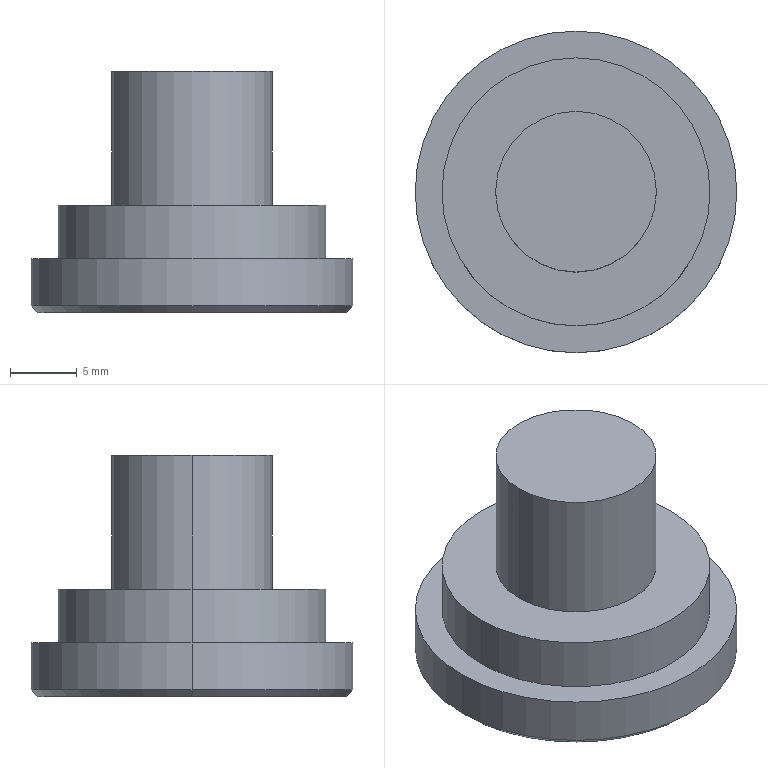Part | SolidWorks | features ICE 2, Chamfer 1, Extrusion 1 | 1 solid | 12 faces | box 24 x 24 x 18 mm | volume 4188 mm3 | cylinder 6 | plane 4 | cone 2 | commonest cylinder face diameters 12 x2 20 x2 24 x2
STEP:
#1=CARTESIAN_POINT('',(-11.5,0.,0.));
#2=VERTEX_POINT('',#1);
#3=CARTESIAN_POINT('',(11.5,0.,0.));
#4=VERTEX_POINT('',#3);
#5=CARTESIAN_POINT('',(0.,0.,0.));
#6=DIRECTION('',(0.,0.,-1.));
#7=DIRECTION('',(1.,0.,0.));
#8=AXIS2_PLACEMENT_3D('',#5,#6,#7);
#9=CIRCLE('',#8,11.5);
#10=EDGE_CURVE('',#2,#4,#9,.T.);
#11=ORIENTED_EDGE('',*,*,#10,.F.);
#12=CARTESIAN_POINT('',(-12.,0.,0.5));
#13=VERTEX_POINT('',#12);
#14=CARTESIAN_POINT('',(-12.,0.,0.5));
#15=DIRECTION('',(-0.7071,0.,0.7071));
#16=VECTOR('',#15,1000.);
#17=LINE('',#14,#16);
#18=EDGE_CURVE('',#2,#13,#17,.T.);
#19=ORIENTED_EDGE('',*,*,#18,.T.);
#20=CARTESIAN_POINT('',(12.,0.,0.5));
#21=VERTEX_POINT('',#20);
#22=CARTESIAN_POINT('',(0.,0.,0.5));
#23=DIRECTION('',(0.,0.,1.));
#24=DIRECTION('',(1.,0.,0.));
#25=AXIS2_PLACEMENT_3D('',#22,#23,#24);
#26=CIRCLE('',#25,12.);
#27=EDGE_CURVE('',#21,#13,#26,.T.);
#28=ORIENTED_EDGE('',*,*,#27,.F.);
#29=CARTESIAN_POINT('',(12.,0.,0.5));
#30=DIRECTION('',(0.7071,0.,0.7071));
#31=VECTOR('',#30,1000.);
#32=LINE('',#29,#31);
#33=EDGE_CURVE('',#4,#21,#32,.T.);
#34=ORIENTED_EDGE('',*,*,#33,.F.);
#35=EDGE_LOOP('',(#11,#19,#28,#34));
#36=FACE_OUTER_BOUND('',#35,.T.);
#37=CARTESIAN_POINT('',(0.,0.,0.5));
#38=DIRECTION('',(0.,0.,1.));
#39=DIRECTION('',(1.,0.,0.));
#40=AXIS2_PLACEMENT_3D('',#37,#38,#39);
#41=CONICAL_SURFACE('',#40,12.,0.7854);
#42=ADVANCED_FACE('',(#36),#41,.T.);
#43=CARTESIAN_POINT('',(12.,0.,4.));
#44=VERTEX_POINT('',#43);
#45=CARTESIAN_POINT('',(-12.,0.,4.));
#46=VERTEX_POINT('',#45);
#47=CARTESIAN_POINT('',(0.,0.,4.));
#48=DIRECTION('',(0.,0.,1.));
#49=DIRECTION('',(1.,0.,0.));
#50=AXIS2_PLACEMENT_3D('',#47,#48,#49);
#51=CIRCLE('',#50,12.);
#52=EDGE_CURVE('',#44,#46,#51,.T.);
#53=ORIENTED_EDGE('',*,*,#52,.F.);
#54=CARTESIAN_POINT('',(12.,0.,4.));
#55=DIRECTION('',(0.,0.,-1.));
#56=VECTOR('',#55,1000.);
#57=LINE('',#54,#56);
#58=EDGE_CURVE('',#44,#21,#57,.T.);
#59=ORIENTED_EDGE('',*,*,#58,.T.);
#60=ORIENTED_EDGE('',*,*,#27,.T.);
#61=CARTESIAN_POINT('',(-12.,0.,4.));
#62=DIRECTION('',(0.,0.,-1.));
#63=VECTOR('',#62,1000.);
#64=LINE('',#61,#63);
#65=EDGE_CURVE('',#46,#13,#64,.T.);
#66=ORIENTED_EDGE('',*,*,#65,.F.);
#67=EDGE_LOOP('',(#53,#59,#60,#66));
#68=FACE_OUTER_BOUND('',#67,.T.);
#69=CARTESIAN_POINT('',(0.,0.,4.));
#70=DIRECTION('',(0.,0.,-1.));
#71=DIRECTION('',(-1.,0.,0.));
#72=AXIS2_PLACEMENT_3D('',#69,#70,#71);
#73=CYLINDRICAL_SURFACE('',#72,12.);
#74=ADVANCED_FACE('',(#68),#73,.T.);
#75=CARTESIAN_POINT('',(10.,0.,8.));
#76=VERTEX_POINT('',#75);
#77=CARTESIAN_POINT('',(-10.,0.,8.));
#78=VERTEX_POINT('',#77);
#79=CARTESIAN_POINT('',(0.,0.,8.));
#80=DIRECTION('',(0.,0.,1.));
#81=DIRECTION('',(1.,0.,0.));
#82=AXIS2_PLACEMENT_3D('',#79,#80,#81);
#83=CIRCLE('',#82,10.);
#84=EDGE_CURVE('',#76,#78,#83,.T.);
#85=ORIENTED_EDGE('',*,*,#84,.F.);
#86=CARTESIAN_POINT('',(10.,0.,4.));
#87=VERTEX_POINT('',#86);
#88=CARTESIAN_POINT('',(10.,0.,8.));
#89=DIRECTION('',(0.,0.,-1.));
#90=VECTOR('',#89,1000.);
#91=LINE('',#88,#90);
#92=EDGE_CURVE('',#76,#87,#91,.T.);
#93=ORIENTED_EDGE('',*,*,#92,.T.);
#94=CARTESIAN_POINT('',(-10.,0.,4.));
#95=VERTEX_POINT('',#94);
#96=CARTESIAN_POINT('',(0.,0.,4.));
#97=DIRECTION('',(0.,0.,1.));
#98=DIRECTION('',(1.,0.,0.));
#99=AXIS2_PLACEMENT_3D('',#96,#97,#98);
#100=CIRCLE('',#99,10.);
#101=EDGE_CURVE('',#87,#95,#100,.T.);
#102=ORIENTED_EDGE('',*,*,#101,.T.);
#103=CARTESIAN_POINT('',(-10.,0.,8.));
#104=DIRECTION('',(0.,0.,-1.));
#105=VECTOR('',#104,1000.);
#106=LINE('',#103,#105);
#107=EDGE_CURVE('',#78,#95,#106,.T.);
#108=ORIENTED_EDGE('',*,*,#107,.F.);
#109=EDGE_LOOP('',(#85,#93,#102,#108));
#110=FACE_OUTER_BOUND('',#109,.T.);
#111=CARTESIAN_POINT('',(0.,0.,8.));
#112=DIRECTION('',(0.,0.,-1.));
#113=DIRECTION('',(-1.,0.,0.));
#114=AXIS2_PLACEMENT_3D('',#111,#112,#113);
#115=CYLINDRICAL_SURFACE('',#114,10.);
#116=ADVANCED_FACE('',(#110),#115,.T.);
#117=CARTESIAN_POINT('',(6.,0.,18.));
#118=VERTEX_POINT('',#117);
#119=CARTESIAN_POINT('',(-6.,0.,18.));
#120=VERTEX_POINT('',#119);
#121=CARTESIAN_POINT('',(0.,0.,18.));
#122=DIRECTION('',(0.,0.,1.));
#123=DIRECTION('',(1.,0.,0.));
#124=AXIS2_PLACEMENT_3D('',#121,#122,#123);
#125=CIRCLE('',#124,6.);
#126=EDGE_CURVE('',#118,#120,#125,.T.);
#127=ORIENTED_EDGE('',*,*,#126,.F.);
#128=CARTESIAN_POINT('',(6.,0.,8.));
#129=VERTEX_POINT('',#128);
#130=CARTESIAN_POINT('',(6.,0.,18.));
#131=DIRECTION('',(0.,0.,-1.));
#132=VECTOR('',#131,1000.);
#133=LINE('',#130,#132);
#134=EDGE_CURVE('',#118,#129,#133,.T.);
#135=ORIENTED_EDGE('',*,*,#134,.T.);
#136=CARTESIAN_POINT('',(-6.,0.,8.));
#137=VERTEX_POINT('',#136);
#138=CARTESIAN_POINT('',(0.,0.,8.));
#139=DIRECTION('',(0.,0.,1.));
#140=DIRECTION('',(1.,0.,0.));
#141=AXIS2_PLACEMENT_3D('',#138,#139,#140);
#142=CIRCLE('',#141,6.);
#143=EDGE_CURVE('',#129,#137,#142,.T.);
#144=ORIENTED_EDGE('',*,*,#143,.T.);
#145=CARTESIAN_POINT('',(-6.,0.,18.));
#146=DIRECTION('',(0.,0.,-1.));
#147=VECTOR('',#146,1000.);
#148=LINE('',#145,#147);
#149=EDGE_CURVE('',#120,#137,#148,.T.);
#150=ORIENTED_EDGE('',*,*,#149,.F.);
#151=EDGE_LOOP('',(#127,#135,#144,#150));
#152=FACE_OUTER_BOUND('',#151,.T.);
#153=CARTESIAN_POINT('',(0.,0.,18.));
#154=DIRECTION('',(0.,0.,-1.));
#155=DIRECTION('',(-1.,0.,0.));
#156=AXIS2_PLACEMENT_3D('',#153,#154,#155);
#157=CYLINDRICAL_SURFACE('',#156,6.);
#158=ADVANCED_FACE('',(#152),#157,.T.);
#159=ORIENTED_EDGE('',*,*,#134,.F.);
#160=CARTESIAN_POINT('',(0.,0.,18.));
#161=DIRECTION('',(0.,0.,1.));
#162=DIRECTION('',(1.,0.,0.));
#163=AXIS2_PLACEMENT_3D('',#160,#161,#162);
#164=CIRCLE('',#163,6.);
#165=EDGE_CURVE('',#120,#118,#164,.T.);
#166=ORIENTED_EDGE('',*,*,#165,.F.);
#167=ORIENTED_EDGE('',*,*,#149,.T.);
#168=CARTESIAN_POINT('',(0.,0.,8.));
#169=DIRECTION('',(0.,0.,1.));
#170=DIRECTION('',(1.,0.,0.));
#171=AXIS2_PLACEMENT_3D('',#168,#169,#170);
#172=CIRCLE('',#171,6.);
#173=EDGE_CURVE('',#137,#129,#172,.T.);
#174=ORIENTED_EDGE('',*,*,#173,.T.);
#175=EDGE_LOOP('',(#159,#166,#167,#174));
#176=FACE_OUTER_BOUND('',#175,.T.);
#177=CARTESIAN_POINT('',(0.,0.,18.));
#178=DIRECTION('',(0.,0.,-1.));
#179=DIRECTION('',(-1.,0.,0.));
#180=AXIS2_PLACEMENT_3D('',#177,#178,#179);
#181=CYLINDRICAL_SURFACE('',#180,6.);
#182=ADVANCED_FACE('',(#176),#181,.T.);
#183=ORIENTED_EDGE('',*,*,#165,.T.);
#184=ORIENTED_EDGE('',*,*,#126,.T.);
#185=EDGE_LOOP('',(#183,#184));
#186=FACE_OUTER_BOUND('',#185,.T.);
#187=CARTESIAN_POINT('',(0.,0.,18.));
#188=DIRECTION('',(0.,0.,1.));
#189=DIRECTION('',(1.,0.,0.));
#190=AXIS2_PLACEMENT_3D('',#187,#188,#189);
#191=PLANE('',#190);
#192=ADVANCED_FACE('',(#186),#191,.T.);
#193=ORIENTED_EDGE('',*,*,#92,.F.);
#194=CARTESIAN_POINT('',(0.,0.,8.));
#195=DIRECTION('',(0.,0.,1.));
#196=DIRECTION('',(1.,0.,0.));
#197=AXIS2_PLACEMENT_3D('',#194,#195,#196);
#198=CIRCLE('',#197,10.);
#199=EDGE_CURVE('',#78,#76,#198,.T.);
#200=ORIENTED_EDGE('',*,*,#199,.F.);
#201=ORIENTED_EDGE('',*,*,#107,.T.);
#202=CARTESIAN_POINT('',(0.,0.,4.));
#203=DIRECTION('',(0.,0.,1.));
#204=DIRECTION('',(1.,0.,0.));
#205=AXIS2_PLACEMENT_3D('',#202,#203,#204);
#206=CIRCLE('',#205,10.);
#207=EDGE_CURVE('',#95,#87,#206,.T.);
#208=ORIENTED_EDGE('',*,*,#207,.T.);
#209=EDGE_LOOP('',(#193,#200,#201,#208));
#210=FACE_OUTER_BOUND('',#209,.T.);
#211=CARTESIAN_POINT('',(0.,0.,8.));
#212=DIRECTION('',(0.,0.,-1.));
#213=DIRECTION('',(-1.,0.,0.));
#214=AXIS2_PLACEMENT_3D('',#211,#212,#213);
#215=CYLINDRICAL_SURFACE('',#214,10.);
#216=ADVANCED_FACE('',(#210),#215,.T.);
#217=ORIENTED_EDGE('',*,*,#173,.F.);
#218=ORIENTED_EDGE('',*,*,#143,.F.);
#219=EDGE_LOOP('',(#217,#218));
#220=FACE_BOUND('',#219,.T.);
#221=ORIENTED_EDGE('',*,*,#199,.T.);
#222=ORIENTED_EDGE('',*,*,#84,.T.);
#223=EDGE_LOOP('',(#221,#222));
#224=FACE_OUTER_BOUND('',#223,.T.);
#225=CARTESIAN_POINT('',(0.,0.,8.));
#226=DIRECTION('',(0.,0.,1.));
#227=DIRECTION('',(1.,0.,0.));
#228=AXIS2_PLACEMENT_3D('',#225,#226,#227);
#229=PLANE('',#228);
#230=ADVANCED_FACE('',(#220,#224),#229,.T.);
#231=ORIENTED_EDGE('',*,*,#58,.F.);
#232=CARTESIAN_POINT('',(0.,0.,4.));
#233=DIRECTION('',(0.,0.,1.));
#234=DIRECTION('',(1.,0.,0.));
#235=AXIS2_PLACEMENT_3D('',#232,#233,#234);
#236=CIRCLE('',#235,12.);
#237=EDGE_CURVE('',#46,#44,#236,.T.);
#238=ORIENTED_EDGE('',*,*,#237,.F.);
#239=ORIENTED_EDGE('',*,*,#65,.T.);
#240=CARTESIAN_POINT('',(0.,0.,0.5));
#241=DIRECTION('',(0.,0.,1.));
#242=DIRECTION('',(1.,0.,0.));
#243=AXIS2_PLACEMENT_3D('',#240,#241,#242);
#244=CIRCLE('',#243,12.);
#245=EDGE_CURVE('',#13,#21,#244,.T.);
#246=ORIENTED_EDGE('',*,*,#245,.T.);
#247=EDGE_LOOP('',(#231,#238,#239,#246));
#248=FACE_OUTER_BOUND('',#247,.T.);
#249=CARTESIAN_POINT('',(0.,0.,4.));
#250=DIRECTION('',(0.,0.,-1.));
#251=DIRECTION('',(-1.,0.,0.));
#252=AXIS2_PLACEMENT_3D('',#249,#250,#251);
#253=CYLINDRICAL_SURFACE('',#252,12.);
#254=ADVANCED_FACE('',(#248),#253,.T.);
#255=ORIENTED_EDGE('',*,*,#207,.F.);
#256=ORIENTED_EDGE('',*,*,#101,.F.);
#257=EDGE_LOOP('',(#255,#256));
#258=FACE_BOUND('',#257,.T.);
#259=ORIENTED_EDGE('',*,*,#237,.T.);
#260=ORIENTED_EDGE('',*,*,#52,.T.);
#261=EDGE_LOOP('',(#259,#260));
#262=FACE_OUTER_BOUND('',#261,.T.);
#263=CARTESIAN_POINT('',(0.,0.,4.));
#264=DIRECTION('',(0.,0.,1.));
#265=DIRECTION('',(1.,0.,0.));
#266=AXIS2_PLACEMENT_3D('',#263,#264,#265);
#267=PLANE('',#266);
#268=ADVANCED_FACE('',(#258,#262),#267,.T.);
#269=CARTESIAN_POINT('',(0.,0.,0.));
#270=DIRECTION('',(0.,0.,-1.));
#271=DIRECTION('',(1.,0.,0.));
#272=AXIS2_PLACEMENT_3D('',#269,#270,#271);
#273=CIRCLE('',#272,11.5);
#274=EDGE_CURVE('',#4,#2,#273,.T.);
#275=ORIENTED_EDGE('',*,*,#274,.T.);
#276=ORIENTED_EDGE('',*,*,#10,.T.);
#277=EDGE_LOOP('',(#275,#276));
#278=FACE_OUTER_BOUND('',#277,.T.);
#279=CARTESIAN_POINT('',(0.,0.,0.));
#280=DIRECTION('',(0.,0.,1.));
#281=DIRECTION('',(1.,0.,0.));
#282=AXIS2_PLACEMENT_3D('',#279,#280,#281);
#283=PLANE('',#282);
#284=ADVANCED_FACE('',(#278),#283,.F.);
#285=ORIENTED_EDGE('',*,*,#18,.F.);
#286=ORIENTED_EDGE('',*,*,#274,.F.);
#287=ORIENTED_EDGE('',*,*,#33,.T.);
#288=ORIENTED_EDGE('',*,*,#245,.F.);
#289=EDGE_LOOP('',(#285,#286,#287,#288));
#290=FACE_OUTER_BOUND('',#289,.T.);
#291=CARTESIAN_POINT('',(0.,0.,0.5));
#292=DIRECTION('',(0.,0.,1.));
#293=DIRECTION('',(1.,0.,0.));
#294=AXIS2_PLACEMENT_3D('',#291,#292,#293);
#295=CONICAL_SURFACE('',#294,12.,0.7854);
#296=ADVANCED_FACE('',(#290),#295,.T.);
#297=CLOSED_SHELL('',(#42,#74,#116,#158,#182,#192,#216,#230,#254,#268,#284,#296));
#298=MANIFOLD_SOLID_BREP('',#297);
#299=CARTESIAN_POINT('',(0.,0.,0.));
#300=DIRECTION('',(0.,0.,1.));
#301=DIRECTION('',(1.,0.,0.));
#302=AXIS2_PLACEMENT_3D('',#299,#300,#301);
#303=(LENGTH_UNIT()NAMED_UNIT(*)SI_UNIT(.MILLI.,.METRE.));
#304=UNCERTAINTY_MEASURE_WITH_UNIT(LENGTH_MEASURE(0.00001),#303,'','');
#305=(NAMED_UNIT(*)PLANE_ANGLE_UNIT()SI_UNIT($,.RADIAN.));
#306=(NAMED_UNIT(*)SI_UNIT($,.STERADIAN.)SOLID_ANGLE_UNIT());
#307=(GEOMETRIC_REPRESENTATION_CONTEXT(3)GLOBAL_UNCERTAINTY_ASSIGNED_CONTEXT((#304))GLOBAL_UNIT_ASSIGNED_CONTEXT((#303,#305,#306))REPRESENTATION_CONTEXT('',''));
#308=ADVANCED_BREP_SHAPE_REPRESENTATION('',(#298,#302),#307);